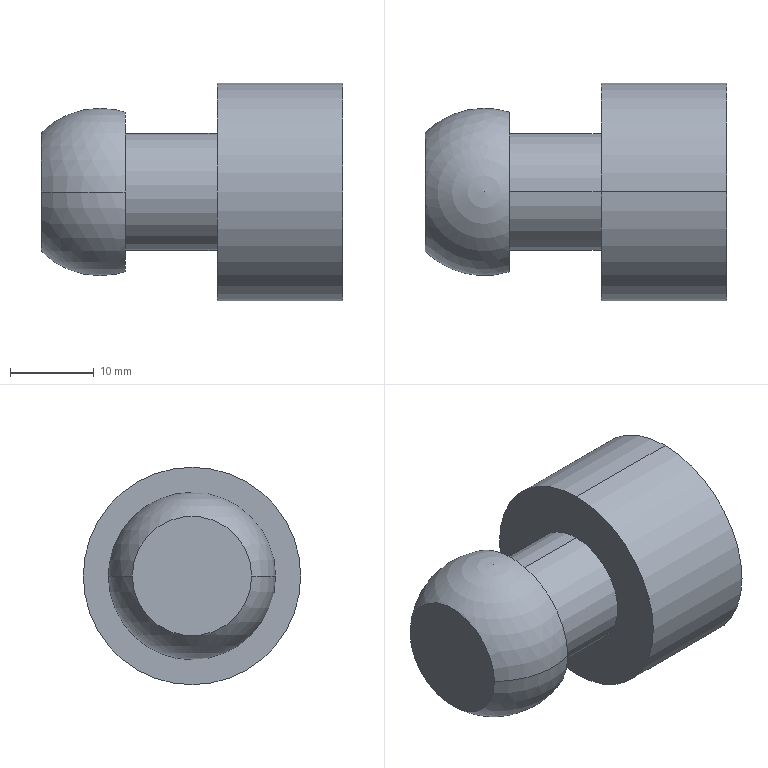Part | SolidWorks | features Revolution 1 | 1 solid | 17 faces | box 36 x 26 x 26 mm | volume 7859 mm3 | cylinder 8 | plane 5 | sphere 2 | cone 2 | commonest cylinder face diameters 10 x2 14 x2 20 x2 26 x2
STEP:
#1=CARTESIAN_POINT('',(0.,0.,-10.));
#2=VERTEX_POINT('',#1);
#3=CARTESIAN_POINT('',(0.,0.,10.));
#4=VERTEX_POINT('',#3);
#5=CARTESIAN_POINT('',(0.,0.,0.));
#6=DIRECTION('',(-1.,0.,0.));
#7=DIRECTION('',(0.,0.,1.));
#8=AXIS2_PLACEMENT_3D('',#5,#6,#7);
#9=CIRCLE('',#8,10.);
#10=EDGE_CURVE('',#2,#4,#9,.T.);
#11=ORIENTED_EDGE('',*,*,#10,.F.);
#12=CARTESIAN_POINT('',(-12.,0.,-10.));
#13=VERTEX_POINT('',#12);
#14=CARTESIAN_POINT('',(0.,0.,-10.));
#15=DIRECTION('',(-1.,0.,0.));
#16=VECTOR('',#15,1000.);
#17=LINE('',#14,#16);
#18=EDGE_CURVE('',#2,#13,#17,.T.);
#19=ORIENTED_EDGE('',*,*,#18,.T.);
#20=CARTESIAN_POINT('',(-12.,0.,10.));
#21=VERTEX_POINT('',#20);
#22=CARTESIAN_POINT('',(-12.,0.,0.));
#23=DIRECTION('',(-1.,0.,0.));
#24=DIRECTION('',(0.,0.,1.));
#25=AXIS2_PLACEMENT_3D('',#22,#23,#24);
#26=CIRCLE('',#25,10.);
#27=EDGE_CURVE('',#13,#21,#26,.T.);
#28=ORIENTED_EDGE('',*,*,#27,.T.);
#29=CARTESIAN_POINT('',(0.,0.,10.));
#30=DIRECTION('',(-1.,0.,0.));
#31=VECTOR('',#30,1000.);
#32=LINE('',#29,#31);
#33=EDGE_CURVE('',#4,#21,#32,.T.);
#34=ORIENTED_EDGE('',*,*,#33,.F.);
#35=EDGE_LOOP('',(#11,#19,#28,#34));
#36=FACE_OUTER_BOUND('',#35,.T.);
#37=CARTESIAN_POINT('',(0.,0.,0.));
#38=DIRECTION('',(-1.,0.,0.));
#39=DIRECTION('',(0.,0.,1.));
#40=AXIS2_PLACEMENT_3D('',#37,#38,#39);
#41=CYLINDRICAL_SURFACE('',#40,10.);
#42=ADVANCED_FACE('',(#36),#41,.F.);
#43=CARTESIAN_POINT('',(0.,0.,13.));
#44=VERTEX_POINT('',#43);
#45=CARTESIAN_POINT('',(0.,0.,-13.));
#46=VERTEX_POINT('',#45);
#47=CARTESIAN_POINT('',(0.,0.,0.));
#48=DIRECTION('',(-1.,0.,0.));
#49=DIRECTION('',(0.,0.,1.));
#50=AXIS2_PLACEMENT_3D('',#47,#48,#49);
#51=CIRCLE('',#50,13.);
#52=EDGE_CURVE('',#44,#46,#51,.T.);
#53=ORIENTED_EDGE('',*,*,#52,.T.);
#54=CARTESIAN_POINT('',(-15.,0.,-13.));
#55=VERTEX_POINT('',#54);
#56=CARTESIAN_POINT('',(0.,0.,-13.));
#57=DIRECTION('',(-1.,0.,0.));
#58=VECTOR('',#57,1000.);
#59=LINE('',#56,#58);
#60=EDGE_CURVE('',#46,#55,#59,.T.);
#61=ORIENTED_EDGE('',*,*,#60,.T.);
#62=CARTESIAN_POINT('',(-15.,0.,13.));
#63=VERTEX_POINT('',#62);
#64=CARTESIAN_POINT('',(-15.,0.,0.));
#65=DIRECTION('',(-1.,0.,0.));
#66=DIRECTION('',(0.,0.,1.));
#67=AXIS2_PLACEMENT_3D('',#64,#65,#66);
#68=CIRCLE('',#67,13.);
#69=EDGE_CURVE('',#63,#55,#68,.T.);
#70=ORIENTED_EDGE('',*,*,#69,.F.);
#71=CARTESIAN_POINT('',(0.,0.,13.));
#72=DIRECTION('',(-1.,0.,0.));
#73=VECTOR('',#72,1000.);
#74=LINE('',#71,#73);
#75=EDGE_CURVE('',#44,#63,#74,.T.);
#76=ORIENTED_EDGE('',*,*,#75,.F.);
#77=EDGE_LOOP('',(#53,#61,#70,#76));
#78=FACE_OUTER_BOUND('',#77,.T.);
#79=CARTESIAN_POINT('',(0.,0.,0.));
#80=DIRECTION('',(-1.,0.,0.));
#81=DIRECTION('',(0.,0.,1.));
#82=AXIS2_PLACEMENT_3D('',#79,#80,#81);
#83=CYLINDRICAL_SURFACE('',#82,13.);
#84=ADVANCED_FACE('',(#78),#83,.T.);
#85=CARTESIAN_POINT('',(-15.,0.,7.));
#86=VERTEX_POINT('',#85);
#87=CARTESIAN_POINT('',(-15.,0.,-7.));
#88=VERTEX_POINT('',#87);
#89=CARTESIAN_POINT('',(-15.,0.,0.));
#90=DIRECTION('',(-1.,0.,0.));
#91=DIRECTION('',(0.,0.,1.));
#92=AXIS2_PLACEMENT_3D('',#89,#90,#91);
#93=CIRCLE('',#92,7.);
#94=EDGE_CURVE('',#86,#88,#93,.T.);
#95=ORIENTED_EDGE('',*,*,#94,.T.);
#96=CARTESIAN_POINT('',(-26.,0.,-7.));
#97=VERTEX_POINT('',#96);
#98=CARTESIAN_POINT('',(0.,0.,-7.));
#99=DIRECTION('',(-1.,0.,0.));
#100=VECTOR('',#99,1000.);
#101=LINE('',#98,#100);
#102=EDGE_CURVE('',#88,#97,#101,.T.);
#103=ORIENTED_EDGE('',*,*,#102,.T.);
#104=CARTESIAN_POINT('',(-26.,0.,7.));
#105=VERTEX_POINT('',#104);
#106=CARTESIAN_POINT('',(-26.,0.,0.));
#107=DIRECTION('',(-1.,0.,0.));
#108=DIRECTION('',(0.,0.,1.));
#109=AXIS2_PLACEMENT_3D('',#106,#107,#108);
#110=CIRCLE('',#109,7.);
#111=EDGE_CURVE('',#105,#97,#110,.T.);
#112=ORIENTED_EDGE('',*,*,#111,.F.);
#113=CARTESIAN_POINT('',(0.,0.,7.));
#114=DIRECTION('',(-1.,0.,0.));
#115=VECTOR('',#114,1000.);
#116=LINE('',#113,#115);
#117=EDGE_CURVE('',#86,#105,#116,.T.);
#118=ORIENTED_EDGE('',*,*,#117,.F.);
#119=EDGE_LOOP('',(#95,#103,#112,#118));
#120=FACE_OUTER_BOUND('',#119,.T.);
#121=CARTESIAN_POINT('',(0.,0.,0.));
#122=DIRECTION('',(-1.,0.,0.));
#123=DIRECTION('',(0.,0.,1.));
#124=AXIS2_PLACEMENT_3D('',#121,#122,#123);
#125=CYLINDRICAL_SURFACE('',#124,7.);
#126=ADVANCED_FACE('',(#120),#125,.T.);
#127=CARTESIAN_POINT('',(-26.,9.539,0.));
#128=VERTEX_POINT('',#127);
#129=CARTESIAN_POINT('',(-26.,-9.539,0.));
#130=VERTEX_POINT('',#129);
#131=CARTESIAN_POINT('',(-26.,0.,0.));
#132=DIRECTION('',(-1.,0.,0.));
#133=DIRECTION('',(0.,0.,1.));
#134=AXIS2_PLACEMENT_3D('',#131,#132,#133);
#135=CIRCLE('',#134,9.539);
#136=EDGE_CURVE('',#128,#130,#135,.T.);
#137=ORIENTED_EDGE('',*,*,#136,.T.);
#138=CARTESIAN_POINT('',(-36.,-7.141,0.));
#139=VERTEX_POINT('',#138);
#140=CARTESIAN_POINT('',(-29.,0.,0.));
#141=DIRECTION('',(0.,0.,-1.));
#142=DIRECTION('',(0.,1.,0.));
#143=AXIS2_PLACEMENT_3D('',#140,#141,#142);
#144=CIRCLE('',#143,10.);
#145=EDGE_CURVE('',#130,#139,#144,.T.);
#146=ORIENTED_EDGE('',*,*,#145,.T.);
#147=CARTESIAN_POINT('',(-36.,7.141,0.));
#148=VERTEX_POINT('',#147);
#149=CARTESIAN_POINT('',(-36.,0.,0.));
#150=DIRECTION('',(-1.,0.,0.));
#151=DIRECTION('',(0.,0.,1.));
#152=AXIS2_PLACEMENT_3D('',#149,#150,#151);
#153=CIRCLE('',#152,7.141);
#154=EDGE_CURVE('',#148,#139,#153,.T.);
#155=ORIENTED_EDGE('',*,*,#154,.F.);
#156=CARTESIAN_POINT('',(-29.,0.,0.));
#157=DIRECTION('',(0.,0.,1.));
#158=DIRECTION('',(1.,0.,0.));
#159=AXIS2_PLACEMENT_3D('',#156,#157,#158);
#160=CIRCLE('',#159,10.);
#161=EDGE_CURVE('',#128,#148,#160,.T.);
#162=ORIENTED_EDGE('',*,*,#161,.F.);
#163=EDGE_LOOP('',(#137,#146,#155,#162));
#164=FACE_OUTER_BOUND('',#163,.T.);
#165=CARTESIAN_POINT('',(-29.,0.,0.));
#166=DIRECTION('',(0.,0.,-1.));
#167=DIRECTION('',(0.,1.,0.));
#168=AXIS2_PLACEMENT_3D('',#165,#166,#167);
#169=SPHERICAL_SURFACE('',#168,10.);
#170=ADVANCED_FACE('',(#164),#169,.T.);
#171=CARTESIAN_POINT('',(-23.887,0.,0.));
#172=VERTEX_POINT('',#171);
#173=CARTESIAN_POINT('',(-21.,0.,-5.));
#174=VERTEX_POINT('',#173);
#175=CARTESIAN_POINT('',(-21.,0.,-5.));
#176=DIRECTION('',(0.5,0.,-0.866));
#177=VECTOR('',#176,1000.);
#178=LINE('',#175,#177);
#179=EDGE_CURVE('',#172,#174,#178,.T.);
#180=ORIENTED_EDGE('',*,*,#179,.F.);
#181=CARTESIAN_POINT('',(-21.,0.,5.));
#182=VERTEX_POINT('',#181);
#183=CARTESIAN_POINT('',(-21.,0.,5.));
#184=DIRECTION('',(0.5,0.,0.866));
#185=VECTOR('',#184,1000.);
#186=LINE('',#183,#185);
#187=EDGE_CURVE('',#172,#182,#186,.T.);
#188=ORIENTED_EDGE('',*,*,#187,.T.);
#189=CARTESIAN_POINT('',(-21.,0.,0.));
#190=DIRECTION('',(-1.,0.,0.));
#191=DIRECTION('',(0.,0.,1.));
#192=AXIS2_PLACEMENT_3D('',#189,#190,#191);
#193=CIRCLE('',#192,5.);
#194=EDGE_CURVE('',#174,#182,#193,.T.);
#195=ORIENTED_EDGE('',*,*,#194,.F.);
#196=EDGE_LOOP('',(#180,#188,#195));
#197=FACE_OUTER_BOUND('',#196,.T.);
#198=CARTESIAN_POINT('',(-21.,0.,0.));
#199=DIRECTION('',(1.,0.,0.));
#200=DIRECTION('',(0.,0.,-1.));
#201=AXIS2_PLACEMENT_3D('',#198,#199,#200);
#202=CONICAL_SURFACE('',#201,5.,1.047);
#203=ADVANCED_FACE('',(#197),#202,.F.);
#204=CARTESIAN_POINT('',(-12.,0.,-5.));
#205=VERTEX_POINT('',#204);
#206=CARTESIAN_POINT('',(-12.,0.,5.));
#207=VERTEX_POINT('',#206);
#208=CARTESIAN_POINT('',(-12.,0.,0.));
#209=DIRECTION('',(-1.,0.,0.));
#210=DIRECTION('',(0.,0.,1.));
#211=AXIS2_PLACEMENT_3D('',#208,#209,#210);
#212=CIRCLE('',#211,5.);
#213=EDGE_CURVE('',#205,#207,#212,.T.);
#214=ORIENTED_EDGE('',*,*,#213,.F.);
#215=CARTESIAN_POINT('',(0.,0.,-5.));
#216=DIRECTION('',(-1.,0.,0.));
#217=VECTOR('',#216,1000.);
#218=LINE('',#215,#217);
#219=EDGE_CURVE('',#205,#174,#218,.T.);
#220=ORIENTED_EDGE('',*,*,#219,.T.);
#221=ORIENTED_EDGE('',*,*,#194,.T.);
#222=CARTESIAN_POINT('',(0.,0.,5.));
#223=DIRECTION('',(-1.,0.,0.));
#224=VECTOR('',#223,1000.);
#225=LINE('',#222,#224);
#226=EDGE_CURVE('',#207,#182,#225,.T.);
#227=ORIENTED_EDGE('',*,*,#226,.F.);
#228=EDGE_LOOP('',(#214,#220,#221,#227));
#229=FACE_OUTER_BOUND('',#228,.T.);
#230=CARTESIAN_POINT('',(0.,0.,0.));
#231=DIRECTION('',(-1.,0.,0.));
#232=DIRECTION('',(0.,0.,1.));
#233=AXIS2_PLACEMENT_3D('',#230,#231,#232);
#234=CYLINDRICAL_SURFACE('',#233,5.);
#235=ADVANCED_FACE('',(#229),#234,.F.);
#236=ORIENTED_EDGE('',*,*,#219,.F.);
#237=CARTESIAN_POINT('',(-12.,0.,0.));
#238=DIRECTION('',(-1.,0.,0.));
#239=DIRECTION('',(0.,0.,1.));
#240=AXIS2_PLACEMENT_3D('',#237,#238,#239);
#241=CIRCLE('',#240,5.);
#242=EDGE_CURVE('',#207,#205,#241,.T.);
#243=ORIENTED_EDGE('',*,*,#242,.F.);
#244=ORIENTED_EDGE('',*,*,#226,.T.);
#245=CARTESIAN_POINT('',(-21.,0.,0.));
#246=DIRECTION('',(-1.,0.,0.));
#247=DIRECTION('',(0.,0.,1.));
#248=AXIS2_PLACEMENT_3D('',#245,#246,#247);
#249=CIRCLE('',#248,5.);
#250=EDGE_CURVE('',#182,#174,#249,.T.);
#251=ORIENTED_EDGE('',*,*,#250,.T.);
#252=EDGE_LOOP('',(#236,#243,#244,#251));
#253=FACE_OUTER_BOUND('',#252,.T.);
#254=CARTESIAN_POINT('',(0.,0.,0.));
#255=DIRECTION('',(-1.,0.,0.));
#256=DIRECTION('',(0.,0.,1.));
#257=AXIS2_PLACEMENT_3D('',#254,#255,#256);
#258=CYLINDRICAL_SURFACE('',#257,5.);
#259=ADVANCED_FACE('',(#253),#258,.F.);
#260=ORIENTED_EDGE('',*,*,#187,.F.);
#261=ORIENTED_EDGE('',*,*,#179,.T.);
#262=ORIENTED_EDGE('',*,*,#250,.F.);
#263=EDGE_LOOP('',(#260,#261,#262));
#264=FACE_OUTER_BOUND('',#263,.T.);
#265=CARTESIAN_POINT('',(-21.,0.,0.));
#266=DIRECTION('',(1.,0.,0.));
#267=DIRECTION('',(0.,0.,-1.));
#268=AXIS2_PLACEMENT_3D('',#265,#266,#267);
#269=CONICAL_SURFACE('',#268,5.,1.047);
#270=ADVANCED_FACE('',(#264),#269,.F.);
#271=ORIENTED_EDGE('',*,*,#154,.T.);
#272=CARTESIAN_POINT('',(-36.,0.,0.));
#273=DIRECTION('',(-1.,0.,0.));
#274=DIRECTION('',(0.,0.,1.));
#275=AXIS2_PLACEMENT_3D('',#272,#273,#274);
#276=CIRCLE('',#275,7.141);
#277=EDGE_CURVE('',#139,#148,#276,.T.);
#278=ORIENTED_EDGE('',*,*,#277,.T.);
#279=EDGE_LOOP('',(#271,#278));
#280=FACE_OUTER_BOUND('',#279,.T.);
#281=CARTESIAN_POINT('',(-36.,0.,0.));
#282=DIRECTION('',(-1.,0.,0.));
#283=DIRECTION('',(0.,0.,1.));
#284=AXIS2_PLACEMENT_3D('',#281,#282,#283);
#285=PLANE('',#284);
#286=ADVANCED_FACE('',(#280),#285,.T.);
#287=ORIENTED_EDGE('',*,*,#145,.F.);
#288=CARTESIAN_POINT('',(-26.,0.,0.));
#289=DIRECTION('',(-1.,0.,0.));
#290=DIRECTION('',(0.,0.,1.));
#291=AXIS2_PLACEMENT_3D('',#288,#289,#290);
#292=CIRCLE('',#291,9.539);
#293=EDGE_CURVE('',#130,#128,#292,.T.);
#294=ORIENTED_EDGE('',*,*,#293,.T.);
#295=ORIENTED_EDGE('',*,*,#161,.T.);
#296=ORIENTED_EDGE('',*,*,#277,.F.);
#297=EDGE_LOOP('',(#287,#294,#295,#296));
#298=FACE_OUTER_BOUND('',#297,.T.);
#299=CARTESIAN_POINT('',(-29.,0.,0.));
#300=DIRECTION('',(0.,0.,-1.));
#301=DIRECTION('',(0.,1.,0.));
#302=AXIS2_PLACEMENT_3D('',#299,#300,#301);
#303=SPHERICAL_SURFACE('',#302,10.);
#304=ADVANCED_FACE('',(#298),#303,.T.);
#305=ORIENTED_EDGE('',*,*,#111,.T.);
#306=CARTESIAN_POINT('',(-26.,0.,0.));
#307=DIRECTION('',(-1.,0.,0.));
#308=DIRECTION('',(0.,0.,1.));
#309=AXIS2_PLACEMENT_3D('',#306,#307,#308);
#310=CIRCLE('',#309,7.);
#311=EDGE_CURVE('',#97,#105,#310,.T.);
#312=ORIENTED_EDGE('',*,*,#311,.T.);
#313=EDGE_LOOP('',(#305,#312));
#314=FACE_BOUND('',#313,.T.);
#315=ORIENTED_EDGE('',*,*,#136,.F.);
#316=ORIENTED_EDGE('',*,*,#293,.F.);
#317=EDGE_LOOP('',(#315,#316));
#318=FACE_OUTER_BOUND('',#317,.T.);
#319=CARTESIAN_POINT('',(-26.,9.539,0.));
#320=DIRECTION('',(1.,0.,0.));
#321=DIRECTION('',(0.,0.,-1.));
#322=AXIS2_PLACEMENT_3D('',#319,#320,#321);
#323=PLANE('',#322);
#324=ADVANCED_FACE('',(#314,#318),#323,.T.);
#325=ORIENTED_EDGE('',*,*,#102,.F.);
#326=CARTESIAN_POINT('',(-15.,0.,0.));
#327=DIRECTION('',(-1.,0.,0.));
#328=DIRECTION('',(0.,0.,1.));
#329=AXIS2_PLACEMENT_3D('',#326,#327,#328);
#330=CIRCLE('',#329,7.);
#331=EDGE_CURVE('',#88,#86,#330,.T.);
#332=ORIENTED_EDGE('',*,*,#331,.T.);
#333=ORIENTED_EDGE('',*,*,#117,.T.);
#334=ORIENTED_EDGE('',*,*,#311,.F.);
#335=EDGE_LOOP('',(#325,#332,#333,#334));
#336=FACE_OUTER_BOUND('',#335,.T.);
#337=CARTESIAN_POINT('',(0.,0.,0.));
#338=DIRECTION('',(-1.,0.,0.));
#339=DIRECTION('',(0.,0.,1.));
#340=AXIS2_PLACEMENT_3D('',#337,#338,#339);
#341=CYLINDRICAL_SURFACE('',#340,7.);
#342=ADVANCED_FACE('',(#336),#341,.T.);
#343=ORIENTED_EDGE('',*,*,#69,.T.);
#344=CARTESIAN_POINT('',(-15.,0.,0.));
#345=DIRECTION('',(-1.,0.,0.));
#346=DIRECTION('',(0.,0.,1.));
#347=AXIS2_PLACEMENT_3D('',#344,#345,#346);
#348=CIRCLE('',#347,13.);
#349=EDGE_CURVE('',#55,#63,#348,.T.);
#350=ORIENTED_EDGE('',*,*,#349,.T.);
#351=EDGE_LOOP('',(#343,#350));
#352=FACE_OUTER_BOUND('',#351,.T.);
#353=ORIENTED_EDGE('',*,*,#94,.F.);
#354=ORIENTED_EDGE('',*,*,#331,.F.);
#355=EDGE_LOOP('',(#353,#354));
#356=FACE_BOUND('',#355,.T.);
#357=CARTESIAN_POINT('',(-15.,7.,0.));
#358=DIRECTION('',(-1.,0.,0.));
#359=DIRECTION('',(0.,0.,1.));
#360=AXIS2_PLACEMENT_3D('',#357,#358,#359);
#361=PLANE('',#360);
#362=ADVANCED_FACE('',(#352,#356),#361,.T.);
#363=ORIENTED_EDGE('',*,*,#60,.F.);
#364=CARTESIAN_POINT('',(0.,0.,0.));
#365=DIRECTION('',(-1.,0.,0.));
#366=DIRECTION('',(0.,0.,1.));
#367=AXIS2_PLACEMENT_3D('',#364,#365,#366);
#368=CIRCLE('',#367,13.);
#369=EDGE_CURVE('',#46,#44,#368,.T.);
#370=ORIENTED_EDGE('',*,*,#369,.T.);
#371=ORIENTED_EDGE('',*,*,#75,.T.);
#372=ORIENTED_EDGE('',*,*,#349,.F.);
#373=EDGE_LOOP('',(#363,#370,#371,#372));
#374=FACE_OUTER_BOUND('',#373,.T.);
#375=CARTESIAN_POINT('',(0.,0.,0.));
#376=DIRECTION('',(-1.,0.,0.));
#377=DIRECTION('',(0.,0.,1.));
#378=AXIS2_PLACEMENT_3D('',#375,#376,#377);
#379=CYLINDRICAL_SURFACE('',#378,13.);
#380=ADVANCED_FACE('',(#374),#379,.T.);
#381=CARTESIAN_POINT('',(0.,0.,0.));
#382=DIRECTION('',(-1.,0.,0.));
#383=DIRECTION('',(0.,0.,1.));
#384=AXIS2_PLACEMENT_3D('',#381,#382,#383);
#385=CIRCLE('',#384,10.);
#386=EDGE_CURVE('',#4,#2,#385,.T.);
#387=ORIENTED_EDGE('',*,*,#386,.T.);
#388=ORIENTED_EDGE('',*,*,#10,.T.);
#389=EDGE_LOOP('',(#387,#388));
#390=FACE_BOUND('',#389,.T.);
#391=ORIENTED_EDGE('',*,*,#52,.F.);
#392=ORIENTED_EDGE('',*,*,#369,.F.);
#393=EDGE_LOOP('',(#391,#392));
#394=FACE_OUTER_BOUND('',#393,.T.);
#395=CARTESIAN_POINT('',(0.,13.,0.));
#396=DIRECTION('',(1.,0.,0.));
#397=DIRECTION('',(0.,0.,-1.));
#398=AXIS2_PLACEMENT_3D('',#395,#396,#397);
#399=PLANE('',#398);
#400=ADVANCED_FACE('',(#390,#394),#399,.T.);
#401=ORIENTED_EDGE('',*,*,#18,.F.);
#402=ORIENTED_EDGE('',*,*,#386,.F.);
#403=ORIENTED_EDGE('',*,*,#33,.T.);
#404=CARTESIAN_POINT('',(-12.,0.,0.));
#405=DIRECTION('',(-1.,0.,0.));
#406=DIRECTION('',(0.,0.,1.));
#407=AXIS2_PLACEMENT_3D('',#404,#405,#406);
#408=CIRCLE('',#407,10.);
#409=EDGE_CURVE('',#21,#13,#408,.T.);
#410=ORIENTED_EDGE('',*,*,#409,.T.);
#411=EDGE_LOOP('',(#401,#402,#403,#410));
#412=FACE_OUTER_BOUND('',#411,.T.);
#413=CARTESIAN_POINT('',(0.,0.,0.));
#414=DIRECTION('',(-1.,0.,0.));
#415=DIRECTION('',(0.,0.,1.));
#416=AXIS2_PLACEMENT_3D('',#413,#414,#415);
#417=CYLINDRICAL_SURFACE('',#416,10.);
#418=ADVANCED_FACE('',(#412),#417,.F.);
#419=ORIENTED_EDGE('',*,*,#242,.T.);
#420=ORIENTED_EDGE('',*,*,#213,.T.);
#421=EDGE_LOOP('',(#419,#420));
#422=FACE_BOUND('',#421,.T.);
#423=ORIENTED_EDGE('',*,*,#409,.F.);
#424=ORIENTED_EDGE('',*,*,#27,.F.);
#425=EDGE_LOOP('',(#423,#424));
#426=FACE_OUTER_BOUND('',#425,.T.);
#427=CARTESIAN_POINT('',(-12.,10.,0.));
#428=DIRECTION('',(1.,0.,0.));
#429=DIRECTION('',(0.,0.,-1.));
#430=AXIS2_PLACEMENT_3D('',#427,#428,#429);
#431=PLANE('',#430);
#432=ADVANCED_FACE('',(#422,#426),#431,.T.);
#433=CLOSED_SHELL('',(#42,#84,#126,#170,#203,#235,#259,#270,#286,#304,#324,#342,#362,#380,#400,#418,#432));
#434=MANIFOLD_SOLID_BREP('',#433);
#435=CARTESIAN_POINT('',(0.,0.,0.));
#436=DIRECTION('',(0.,0.,1.));
#437=DIRECTION('',(1.,0.,0.));
#438=AXIS2_PLACEMENT_3D('',#435,#436,#437);
#439=(LENGTH_UNIT()NAMED_UNIT(*)SI_UNIT(.MILLI.,.METRE.));
#440=UNCERTAINTY_MEASURE_WITH_UNIT(LENGTH_MEASURE(0.00001),#439,'','');
#441=(NAMED_UNIT(*)PLANE_ANGLE_UNIT()SI_UNIT($,.RADIAN.));
#442=(NAMED_UNIT(*)SI_UNIT($,.STERADIAN.)SOLID_ANGLE_UNIT());
#443=(GEOMETRIC_REPRESENTATION_CONTEXT(3)GLOBAL_UNCERTAINTY_ASSIGNED_CONTEXT((#440))GLOBAL_UNIT_ASSIGNED_CONTEXT((#439,#441,#442))REPRESENTATION_CONTEXT('',''));
#444=ADVANCED_BREP_SHAPE_REPRESENTATION('',(#434,#438),#443);